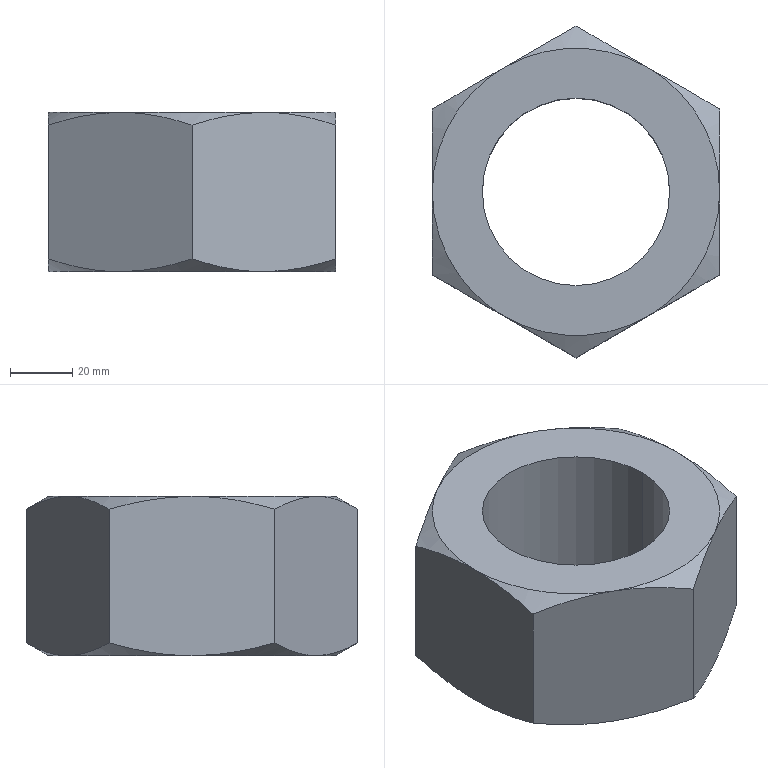Part | SolidWorks | features BaseBody 1 | 1 solid | 22 faces | box 92 x 106.232 x 51 mm | volume 227942 mm3 | cone 12 | plane 8 | cylinder 2 | commonest cylinder face diameters 60 x2
STEP:
#1=CARTESIAN_POINT('',(-30.,0.,51.));
#2=VERTEX_POINT('',#1);
#3=CARTESIAN_POINT('',(30.,0.,51.));
#4=VERTEX_POINT('',#3);
#5=CARTESIAN_POINT('',(0.,0.,51.));
#6=DIRECTION('',(0.,0.,1.));
#7=DIRECTION('',(1.,0.,0.));
#8=AXIS2_PLACEMENT_3D('',#5,#6,#7);
#9=CIRCLE('',#8,30.);
#10=EDGE_CURVE('',#2,#4,#9,.T.);
#11=ORIENTED_EDGE('',*,*,#10,.T.);
#12=CARTESIAN_POINT('',(30.,0.,0.));
#13=VERTEX_POINT('',#12);
#14=CARTESIAN_POINT('',(30.,0.,51.));
#15=DIRECTION('',(0.,0.,-1.));
#16=VECTOR('',#15,1000.);
#17=LINE('',#14,#16);
#18=EDGE_CURVE('',#4,#13,#17,.T.);
#19=ORIENTED_EDGE('',*,*,#18,.T.);
#20=CARTESIAN_POINT('',(-30.,0.,0.));
#21=VERTEX_POINT('',#20);
#22=CARTESIAN_POINT('',(0.,0.,0.));
#23=DIRECTION('',(0.,0.,1.));
#24=DIRECTION('',(1.,0.,0.));
#25=AXIS2_PLACEMENT_3D('',#22,#23,#24);
#26=CIRCLE('',#25,30.);
#27=EDGE_CURVE('',#21,#13,#26,.T.);
#28=ORIENTED_EDGE('',*,*,#27,.F.);
#29=CARTESIAN_POINT('',(-30.,0.,51.));
#30=DIRECTION('',(0.,0.,-1.));
#31=VECTOR('',#30,1000.);
#32=LINE('',#29,#31);
#33=EDGE_CURVE('',#2,#21,#32,.T.);
#34=ORIENTED_EDGE('',*,*,#33,.F.);
#35=EDGE_LOOP('',(#11,#19,#28,#34));
#36=FACE_OUTER_BOUND('',#35,.T.);
#37=CARTESIAN_POINT('',(0.,0.,51.));
#38=DIRECTION('',(0.,0.,-1.));
#39=DIRECTION('',(-1.,0.,0.));
#40=AXIS2_PLACEMENT_3D('',#37,#38,#39);
#41=CYLINDRICAL_SURFACE('',#40,30.);
#42=ADVANCED_FACE('',(#36),#41,.F.);
#43=CARTESIAN_POINT('',(46.,26.558,46.891));
#44=VERTEX_POINT('',#43);
#45=CARTESIAN_POINT('',(23.,39.837,51.));
#46=VERTEX_POINT('',#45);
#47=CARTESIAN_POINT('',(46.,26.558,46.891));
#48=CARTESIAN_POINT('',(42.237,28.73,48.146));
#49=CARTESIAN_POINT('',(38.448,30.919,49.179));
#50=CARTESIAN_POINT('',(32.703,34.235,50.251));
#51=CARTESIAN_POINT('',(30.778,35.346,50.529));
#52=CARTESIAN_POINT('',(26.906,37.582,50.903));
#53=CARTESIAN_POINT('',(24.959,38.706,51.));
#54=CARTESIAN_POINT('',(23.,39.837,51.));
#55=B_SPLINE_CURVE_WITH_KNOTS('',3,(#47,#48,#49,#50,#51,#52,#53,#54),.UNSPECIFIED.,.F.,.F.,(4,2,2,4),(0.000000238,0.01344,0.02015,0.02687),.UNSPECIFIED.);
#56=EDGE_CURVE('',#44,#46,#55,.T.);
#57=ORIENTED_EDGE('',*,*,#56,.F.);
#58=CARTESIAN_POINT('',(46.,26.558,4.109));
#59=VERTEX_POINT('',#58);
#60=CARTESIAN_POINT('',(46.,26.558,51.));
#61=DIRECTION('',(0.,0.,-1.));
#62=VECTOR('',#61,1000.);
#63=LINE('',#60,#62);
#64=EDGE_CURVE('',#44,#59,#63,.T.);
#65=ORIENTED_EDGE('',*,*,#64,.T.);
#66=CARTESIAN_POINT('',(23.,39.837,0.));
#67=VERTEX_POINT('',#66);
#68=CARTESIAN_POINT('',(23.,39.837,0.));
#69=CARTESIAN_POINT('',(23.976,39.274,0.));
#70=CARTESIAN_POINT('',(24.957,38.707,0.0241));
#71=CARTESIAN_POINT('',(26.909,37.58,0.1197));
#72=CARTESIAN_POINT('',(27.882,37.018,0.1911));
#73=CARTESIAN_POINT('',(30.791,35.339,0.4729));
#74=CARTESIAN_POINT('',(32.718,34.227,0.7513));
#75=CARTESIAN_POINT('',(38.462,30.91,1.825));
#76=CARTESIAN_POINT('',(42.247,28.725,2.858));
#77=CARTESIAN_POINT('',(46.,26.558,4.109));
#78=B_SPLINE_CURVE_WITH_KNOTS('',3,(#68,#69,#70,#71,#72,#73,#74,#75,#76,#77),.UNSPECIFIED.,.F.,.F.,(4,2,2,2,4),(0.02687,0.03022,0.03357,0.04026,0.05364),.UNSPECIFIED.);
#79=EDGE_CURVE('',#67,#59,#78,.T.);
#80=ORIENTED_EDGE('',*,*,#79,.F.);
#81=CARTESIAN_POINT('',(0.,53.116,4.109));
#82=VERTEX_POINT('',#81);
#83=CARTESIAN_POINT('',(0.,53.116,4.109));
#84=CARTESIAN_POINT('',(3.763,50.944,2.854));
#85=CARTESIAN_POINT('',(7.552,48.756,1.821));
#86=CARTESIAN_POINT('',(13.297,45.439,0.749));
#87=CARTESIAN_POINT('',(15.222,44.328,0.4714));
#88=CARTESIAN_POINT('',(19.094,42.093,0.09681));
#89=CARTESIAN_POINT('',(21.041,40.968,0.));
#90=CARTESIAN_POINT('',(23.,39.837,0.));
#91=B_SPLINE_CURVE_WITH_KNOTS('',3,(#83,#84,#85,#86,#87,#88,#89,#90),.UNSPECIFIED.,.F.,.F.,(4,2,2,4),(0.000000238,0.01344,0.02015,0.02687),.UNSPECIFIED.);
#92=EDGE_CURVE('',#82,#67,#91,.T.);
#93=ORIENTED_EDGE('',*,*,#92,.F.);
#94=CARTESIAN_POINT('',(0.,53.116,46.891));
#95=VERTEX_POINT('',#94);
#96=CARTESIAN_POINT('',(0.,53.116,51.));
#97=DIRECTION('',(0.,0.,-1.));
#98=VECTOR('',#97,1000.);
#99=LINE('',#96,#98);
#100=EDGE_CURVE('',#95,#82,#99,.T.);
#101=ORIENTED_EDGE('',*,*,#100,.F.);
#102=CARTESIAN_POINT('',(23.,39.837,51.));
#103=CARTESIAN_POINT('',(22.024,40.401,51.));
#104=CARTESIAN_POINT('',(21.043,40.967,50.976));
#105=CARTESIAN_POINT('',(19.091,42.094,50.88));
#106=CARTESIAN_POINT('',(18.118,42.656,50.809));
#107=CARTESIAN_POINT('',(15.209,44.335,50.527));
#108=CARTESIAN_POINT('',(13.282,45.448,50.249));
#109=CARTESIAN_POINT('',(7.538,48.764,49.175));
#110=CARTESIAN_POINT('',(3.753,50.949,48.142));
#111=CARTESIAN_POINT('',(0.,53.116,46.891));
#112=B_SPLINE_CURVE_WITH_KNOTS('',3,(#102,#103,#104,#105,#106,#107,#108,#109,#110,#111),.UNSPECIFIED.,.F.,.F.,(4,2,2,2,4),(0.02687,0.03022,0.03357,0.04026,0.05364),.UNSPECIFIED.);
#113=EDGE_CURVE('',#46,#95,#112,.T.);
#114=ORIENTED_EDGE('',*,*,#113,.F.);
#115=EDGE_LOOP('',(#57,#65,#80,#93,#101,#114));
#116=FACE_OUTER_BOUND('',#115,.T.);
#117=CARTESIAN_POINT('',(46.,26.558,51.));
#118=DIRECTION('',(-0.5,-0.866,0.));
#119=DIRECTION('',(0.866,-0.5,0.));
#120=AXIS2_PLACEMENT_3D('',#117,#118,#119);
#121=PLANE('',#120);
#122=ADVANCED_FACE('',(#116),#121,.F.);
#123=CARTESIAN_POINT('',(-23.,39.837,51.));
#124=VERTEX_POINT('',#123);
#125=CARTESIAN_POINT('',(0.,53.116,46.891));
#126=CARTESIAN_POINT('',(-3.763,50.944,48.146));
#127=CARTESIAN_POINT('',(-7.552,48.756,49.179));
#128=CARTESIAN_POINT('',(-13.297,45.439,50.251));
#129=CARTESIAN_POINT('',(-15.222,44.328,50.529));
#130=CARTESIAN_POINT('',(-19.094,42.093,50.903));
#131=CARTESIAN_POINT('',(-21.041,40.968,51.));
#132=CARTESIAN_POINT('',(-23.,39.837,51.));
#133=B_SPLINE_CURVE_WITH_KNOTS('',3,(#125,#126,#127,#128,#129,#130,#131,#132),.UNSPECIFIED.,.F.,.F.,(4,2,2,4),(0.000000238,0.01344,0.02015,0.02687),.UNSPECIFIED.);
#134=EDGE_CURVE('',#95,#124,#133,.T.);
#135=ORIENTED_EDGE('',*,*,#134,.F.);
#136=ORIENTED_EDGE('',*,*,#100,.T.);
#137=CARTESIAN_POINT('',(-23.,39.837,0.));
#138=VERTEX_POINT('',#137);
#139=CARTESIAN_POINT('',(-23.,39.837,0.));
#140=CARTESIAN_POINT('',(-22.024,40.401,0.));
#141=CARTESIAN_POINT('',(-21.043,40.967,0.0241));
#142=CARTESIAN_POINT('',(-19.091,42.094,0.1197));
#143=CARTESIAN_POINT('',(-18.118,42.656,0.1911));
#144=CARTESIAN_POINT('',(-15.209,44.335,0.4729));
#145=CARTESIAN_POINT('',(-13.282,45.448,0.7513));
#146=CARTESIAN_POINT('',(-7.538,48.764,1.825));
#147=CARTESIAN_POINT('',(-3.753,50.949,2.858));
#148=CARTESIAN_POINT('',(0.,53.116,4.109));
#149=B_SPLINE_CURVE_WITH_KNOTS('',3,(#139,#140,#141,#142,#143,#144,#145,#146,#147,#148),.UNSPECIFIED.,.F.,.F.,(4,2,2,2,4),(0.02687,0.03022,0.03357,0.04026,0.05364),.UNSPECIFIED.);
#150=EDGE_CURVE('',#138,#82,#149,.T.);
#151=ORIENTED_EDGE('',*,*,#150,.F.);
#152=CARTESIAN_POINT('',(-46.,26.558,4.109));
#153=VERTEX_POINT('',#152);
#154=CARTESIAN_POINT('',(-46.,26.558,4.109));
#155=CARTESIAN_POINT('',(-42.237,28.73,2.854));
#156=CARTESIAN_POINT('',(-38.448,30.919,1.821));
#157=CARTESIAN_POINT('',(-32.703,34.235,0.749));
#158=CARTESIAN_POINT('',(-30.778,35.346,0.4714));
#159=CARTESIAN_POINT('',(-26.906,37.582,0.09681));
#160=CARTESIAN_POINT('',(-24.959,38.706,0.));
#161=CARTESIAN_POINT('',(-23.,39.837,0.));
#162=B_SPLINE_CURVE_WITH_KNOTS('',3,(#154,#155,#156,#157,#158,#159,#160,#161),.UNSPECIFIED.,.F.,.F.,(4,2,2,4),(0.000000238,0.01344,0.02015,0.02687),.UNSPECIFIED.);
#163=EDGE_CURVE('',#153,#138,#162,.T.);
#164=ORIENTED_EDGE('',*,*,#163,.F.);
#165=CARTESIAN_POINT('',(-46.,26.558,46.891));
#166=VERTEX_POINT('',#165);
#167=CARTESIAN_POINT('',(-46.,26.558,51.));
#168=DIRECTION('',(0.,0.,-1.));
#169=VECTOR('',#168,1000.);
#170=LINE('',#167,#169);
#171=EDGE_CURVE('',#166,#153,#170,.T.);
#172=ORIENTED_EDGE('',*,*,#171,.F.);
#173=CARTESIAN_POINT('',(-23.,39.837,51.));
#174=CARTESIAN_POINT('',(-23.976,39.274,51.));
#175=CARTESIAN_POINT('',(-24.957,38.707,50.976));
#176=CARTESIAN_POINT('',(-26.909,37.58,50.88));
#177=CARTESIAN_POINT('',(-27.882,37.018,50.809));
#178=CARTESIAN_POINT('',(-30.791,35.339,50.527));
#179=CARTESIAN_POINT('',(-32.718,34.227,50.249));
#180=CARTESIAN_POINT('',(-38.462,30.91,49.175));
#181=CARTESIAN_POINT('',(-42.247,28.725,48.142));
#182=CARTESIAN_POINT('',(-46.,26.558,46.891));
#183=B_SPLINE_CURVE_WITH_KNOTS('',3,(#173,#174,#175,#176,#177,#178,#179,#180,#181,#182),.UNSPECIFIED.,.F.,.F.,(4,2,2,2,4),(0.02687,0.03022,0.03357,0.04026,0.05364),.UNSPECIFIED.);
#184=EDGE_CURVE('',#124,#166,#183,.T.);
#185=ORIENTED_EDGE('',*,*,#184,.F.);
#186=EDGE_LOOP('',(#135,#136,#151,#164,#172,#185));
#187=FACE_OUTER_BOUND('',#186,.T.);
#188=CARTESIAN_POINT('',(0.,53.116,51.));
#189=DIRECTION('',(0.5,-0.866,0.));
#190=DIRECTION('',(0.866,0.5,0.));
#191=AXIS2_PLACEMENT_3D('',#188,#189,#190);
#192=PLANE('',#191);
#193=ADVANCED_FACE('',(#187),#192,.F.);
#194=CARTESIAN_POINT('',(-46.,0.,51.));
#195=VERTEX_POINT('',#194);
#196=CARTESIAN_POINT('',(-46.,26.558,46.891));
#197=CARTESIAN_POINT('',(-46.,22.263,48.131));
#198=CARTESIAN_POINT('',(-46.,17.913,49.163));
#199=CARTESIAN_POINT('',(-46.,11.264,50.243));
#200=CARTESIAN_POINT('',(-46.,9.027,50.524));
#201=CARTESIAN_POINT('',(-46.,4.504,50.904));
#202=CARTESIAN_POINT('',(-46.,2.247,51.));
#203=CARTESIAN_POINT('',(-46.,0.,51.));
#204=B_SPLINE_CURVE_WITH_KNOTS('',3,(#196,#197,#198,#199,#200,#201,#202,#203),.UNSPECIFIED.,.F.,.F.,(4,2,2,4),(0.1492,0.1627,0.1694,0.1761),.UNSPECIFIED.);
#205=EDGE_CURVE('',#166,#195,#204,.T.);
#206=ORIENTED_EDGE('',*,*,#205,.F.);
#207=ORIENTED_EDGE('',*,*,#171,.T.);
#208=CARTESIAN_POINT('',(-46.,0.,0.));
#209=VERTEX_POINT('',#208);
#210=CARTESIAN_POINT('',(-46.,0.,0.));
#211=CARTESIAN_POINT('',(-46.,2.247,0.));
#212=CARTESIAN_POINT('',(-46.,4.504,0.09573));
#213=CARTESIAN_POINT('',(-46.,9.027,0.4757));
#214=CARTESIAN_POINT('',(-46.,11.264,0.757));
#215=CARTESIAN_POINT('',(-46.,17.913,1.837));
#216=CARTESIAN_POINT('',(-46.,22.263,2.869));
#217=CARTESIAN_POINT('',(-46.,26.558,4.109));
#218=B_SPLINE_CURVE_WITH_KNOTS('',3,(#210,#211,#212,#213,#214,#215,#216,#217),.UNSPECIFIED.,.F.,.F.,(4,2,2,4),(0.07541,0.08213,0.08886,0.1023),.UNSPECIFIED.);
#219=EDGE_CURVE('',#209,#153,#218,.T.);
#220=ORIENTED_EDGE('',*,*,#219,.F.);
#221=CARTESIAN_POINT('',(-46.,-26.558,4.109));
#222=VERTEX_POINT('',#221);
#223=CARTESIAN_POINT('',(-46.,-26.558,4.109));
#224=CARTESIAN_POINT('',(-46.,-25.477,3.797));
#225=CARTESIAN_POINT('',(-46.,-24.392,3.497));
#226=CARTESIAN_POINT('',(-46.,-22.209,2.928));
#227=CARTESIAN_POINT('',(-46.,-21.11,2.657));
#228=CARTESIAN_POINT('',(-46.,-17.806,1.896));
#229=CARTESIAN_POINT('',(-46.,-15.597,1.458));
#230=CARTESIAN_POINT('',(-46.,-11.166,0.7436));
#231=CARTESIAN_POINT('',(-46.,-8.943,0.4673));
#232=CARTESIAN_POINT('',(-46.,-4.483,0.09541));
#233=CARTESIAN_POINT('',(-46.,-2.246,0.));
#234=CARTESIAN_POINT('',(-46.,0.,0.));
#235=B_SPLINE_CURVE_WITH_KNOTS('',3,(#223,#224,#225,#226,#227,#228,#229,#230,#231,#232,#233,#234),.UNSPECIFIED.,.F.,.F.,(4,2,2,2,2,4),(0.04853,0.05189,0.05525,0.06197,0.06869,0.07541),.UNSPECIFIED.);
#236=EDGE_CURVE('',#222,#209,#235,.T.);
#237=ORIENTED_EDGE('',*,*,#236,.F.);
#238=CARTESIAN_POINT('',(-46.,-26.558,46.891));
#239=VERTEX_POINT('',#238);
#240=CARTESIAN_POINT('',(-46.,-26.558,51.));
#241=DIRECTION('',(0.,0.,-1.));
#242=VECTOR('',#241,1000.);
#243=LINE('',#240,#242);
#244=EDGE_CURVE('',#239,#222,#243,.T.);
#245=ORIENTED_EDGE('',*,*,#244,.F.);
#246=CARTESIAN_POINT('',(-46.,0.,51.));
#247=CARTESIAN_POINT('',(-46.,-2.246,51.));
#248=CARTESIAN_POINT('',(-46.,-4.483,50.905));
#249=CARTESIAN_POINT('',(-46.,-8.943,50.533));
#250=CARTESIAN_POINT('',(-46.,-11.166,50.256));
#251=CARTESIAN_POINT('',(-46.,-15.597,49.542));
#252=CARTESIAN_POINT('',(-46.,-17.806,49.104));
#253=CARTESIAN_POINT('',(-46.,-21.11,48.343));
#254=CARTESIAN_POINT('',(-46.,-22.209,48.072));
#255=CARTESIAN_POINT('',(-46.,-24.392,47.503));
#256=CARTESIAN_POINT('',(-46.,-25.477,47.203));
#257=CARTESIAN_POINT('',(-46.,-26.558,46.891));
#258=B_SPLINE_CURVE_WITH_KNOTS('',3,(#246,#247,#248,#249,#250,#251,#252,#253,#254,#255,#256,#257),.UNSPECIFIED.,.F.,.F.,(4,2,2,2,2,4),(0.1761,0.1828,0.1895,0.1963,0.1996,0.203),.UNSPECIFIED.);
#259=EDGE_CURVE('',#195,#239,#258,.T.);
#260=ORIENTED_EDGE('',*,*,#259,.F.);
#261=EDGE_LOOP('',(#206,#207,#220,#237,#245,#260));
#262=FACE_OUTER_BOUND('',#261,.T.);
#263=CARTESIAN_POINT('',(-46.,26.558,51.));
#264=DIRECTION('',(1.,0.,0.));
#265=DIRECTION('',(0.,1.,0.));
#266=AXIS2_PLACEMENT_3D('',#263,#264,#265);
#267=PLANE('',#266);
#268=ADVANCED_FACE('',(#262),#267,.F.);
#269=CARTESIAN_POINT('',(-23.,-39.837,51.));
#270=VERTEX_POINT('',#269);
#271=CARTESIAN_POINT('',(-46.,-26.558,46.891));
#272=CARTESIAN_POINT('',(-42.237,-28.73,48.146));
#273=CARTESIAN_POINT('',(-38.448,-30.919,49.179));
#274=CARTESIAN_POINT('',(-32.703,-34.235,50.251));
#275=CARTESIAN_POINT('',(-30.778,-35.346,50.529));
#276=CARTESIAN_POINT('',(-26.906,-37.582,50.903));
#277=CARTESIAN_POINT('',(-24.959,-38.706,51.));
#278=CARTESIAN_POINT('',(-23.,-39.837,51.));
#279=B_SPLINE_CURVE_WITH_KNOTS('',3,(#271,#272,#273,#274,#275,#276,#277,#278),.UNSPECIFIED.,.F.,.F.,(4,2,2,4),(0.000000238,0.01344,0.02015,0.02687),.UNSPECIFIED.);
#280=EDGE_CURVE('',#239,#270,#279,.T.);
#281=ORIENTED_EDGE('',*,*,#280,.F.);
#282=ORIENTED_EDGE('',*,*,#244,.T.);
#283=CARTESIAN_POINT('',(-23.,-39.837,0.));
#284=VERTEX_POINT('',#283);
#285=CARTESIAN_POINT('',(-23.,-39.837,0.));
#286=CARTESIAN_POINT('',(-23.976,-39.274,0.));
#287=CARTESIAN_POINT('',(-24.957,-38.707,0.0241));
#288=CARTESIAN_POINT('',(-26.909,-37.58,0.1197));
#289=CARTESIAN_POINT('',(-27.882,-37.018,0.1911));
#290=CARTESIAN_POINT('',(-30.791,-35.339,0.4729));
#291=CARTESIAN_POINT('',(-32.718,-34.227,0.7513));
#292=CARTESIAN_POINT('',(-38.462,-30.91,1.825));
#293=CARTESIAN_POINT('',(-42.247,-28.725,2.858));
#294=CARTESIAN_POINT('',(-46.,-26.558,4.109));
#295=B_SPLINE_CURVE_WITH_KNOTS('',3,(#285,#286,#287,#288,#289,#290,#291,#292,#293,#294),.UNSPECIFIED.,.F.,.F.,(4,2,2,2,4),(0.02687,0.03022,0.03357,0.04026,0.05364),.UNSPECIFIED.);
#296=EDGE_CURVE('',#284,#222,#295,.T.);
#297=ORIENTED_EDGE('',*,*,#296,.F.);
#298=CARTESIAN_POINT('',(0.,-53.116,4.109));
#299=VERTEX_POINT('',#298);
#300=CARTESIAN_POINT('',(0.,-53.116,4.109));
#301=CARTESIAN_POINT('',(-3.763,-50.944,2.854));
#302=CARTESIAN_POINT('',(-7.552,-48.756,1.821));
#303=CARTESIAN_POINT('',(-13.297,-45.439,0.749));
#304=CARTESIAN_POINT('',(-15.222,-44.328,0.4714));
#305=CARTESIAN_POINT('',(-19.094,-42.093,0.09681));
#306=CARTESIAN_POINT('',(-21.041,-40.968,0.));
#307=CARTESIAN_POINT('',(-23.,-39.837,0.));
#308=B_SPLINE_CURVE_WITH_KNOTS('',3,(#300,#301,#302,#303,#304,#305,#306,#307),.UNSPECIFIED.,.F.,.F.,(4,2,2,4),(0.000000238,0.01344,0.02015,0.02687),.UNSPECIFIED.);
#309=EDGE_CURVE('',#299,#284,#308,.T.);
#310=ORIENTED_EDGE('',*,*,#309,.F.);
#311=CARTESIAN_POINT('',(0.,-53.116,46.891));
#312=VERTEX_POINT('',#311);
#313=CARTESIAN_POINT('',(0.,-53.116,51.));
#314=DIRECTION('',(0.,0.,-1.));
#315=VECTOR('',#314,1000.);
#316=LINE('',#313,#315);
#317=EDGE_CURVE('',#312,#299,#316,.T.);
#318=ORIENTED_EDGE('',*,*,#317,.F.);
#319=CARTESIAN_POINT('',(-23.,-39.837,51.));
#320=CARTESIAN_POINT('',(-22.024,-40.401,51.));
#321=CARTESIAN_POINT('',(-21.043,-40.967,50.976));
#322=CARTESIAN_POINT('',(-19.091,-42.094,50.88));
#323=CARTESIAN_POINT('',(-18.118,-42.656,50.809));
#324=CARTESIAN_POINT('',(-15.209,-44.335,50.527));
#325=CARTESIAN_POINT('',(-13.282,-45.448,50.249));
#326=CARTESIAN_POINT('',(-7.538,-48.764,49.175));
#327=CARTESIAN_POINT('',(-3.753,-50.949,48.142));
#328=CARTESIAN_POINT('',(0.,-53.116,46.891));
#329=B_SPLINE_CURVE_WITH_KNOTS('',3,(#319,#320,#321,#322,#323,#324,#325,#326,#327,#328),.UNSPECIFIED.,.F.,.F.,(4,2,2,2,4),(0.02687,0.03022,0.03357,0.04026,0.05364),.UNSPECIFIED.);
#330=EDGE_CURVE('',#270,#312,#329,.T.);
#331=ORIENTED_EDGE('',*,*,#330,.F.);
#332=EDGE_LOOP('',(#281,#282,#297,#310,#318,#331));
#333=FACE_OUTER_BOUND('',#332,.T.);
#334=CARTESIAN_POINT('',(-46.,-26.558,51.));
#335=DIRECTION('',(0.5,0.866,0.));
#336=DIRECTION('',(-0.866,0.5,0.));
#337=AXIS2_PLACEMENT_3D('',#334,#335,#336);
#338=PLANE('',#337);
#339=ADVANCED_FACE('',(#333),#338,.F.);
#340=CARTESIAN_POINT('',(23.,-39.837,51.));
#341=VERTEX_POINT('',#340);
#342=CARTESIAN_POINT('',(0.,-53.116,46.891));
#343=CARTESIAN_POINT('',(3.763,-50.944,48.146));
#344=CARTESIAN_POINT('',(7.552,-48.756,49.179));
#345=CARTESIAN_POINT('',(13.297,-45.439,50.251));
#346=CARTESIAN_POINT('',(15.222,-44.328,50.529));
#347=CARTESIAN_POINT('',(19.094,-42.093,50.903));
#348=CARTESIAN_POINT('',(21.041,-40.968,51.));
#349=CARTESIAN_POINT('',(23.,-39.837,51.));
#350=B_SPLINE_CURVE_WITH_KNOTS('',3,(#342,#343,#344,#345,#346,#347,#348,#349),.UNSPECIFIED.,.F.,.F.,(4,2,2,4),(0.000000238,0.01344,0.02015,0.02687),.UNSPECIFIED.);
#351=EDGE_CURVE('',#312,#341,#350,.T.);
#352=ORIENTED_EDGE('',*,*,#351,.F.);
#353=ORIENTED_EDGE('',*,*,#317,.T.);
#354=CARTESIAN_POINT('',(23.,-39.837,0.));
#355=VERTEX_POINT('',#354);
#356=CARTESIAN_POINT('',(23.,-39.837,0.));
#357=CARTESIAN_POINT('',(22.024,-40.401,0.));
#358=CARTESIAN_POINT('',(21.043,-40.967,0.0241));
#359=CARTESIAN_POINT('',(19.091,-42.094,0.1197));
#360=CARTESIAN_POINT('',(18.118,-42.656,0.1911));
#361=CARTESIAN_POINT('',(15.209,-44.335,0.4729));
#362=CARTESIAN_POINT('',(13.282,-45.448,0.7513));
#363=CARTESIAN_POINT('',(7.538,-48.764,1.825));
#364=CARTESIAN_POINT('',(3.753,-50.949,2.858));
#365=CARTESIAN_POINT('',(0.,-53.116,4.109));
#366=B_SPLINE_CURVE_WITH_KNOTS('',3,(#356,#357,#358,#359,#360,#361,#362,#363,#364,#365),.UNSPECIFIED.,.F.,.F.,(4,2,2,2,4),(0.02687,0.03022,0.03357,0.04026,0.05364),.UNSPECIFIED.);
#367=EDGE_CURVE('',#355,#299,#366,.T.);
#368=ORIENTED_EDGE('',*,*,#367,.F.);
#369=CARTESIAN_POINT('',(46.,-26.558,4.109));
#370=VERTEX_POINT('',#369);
#371=CARTESIAN_POINT('',(46.,-26.558,4.109));
#372=CARTESIAN_POINT('',(42.237,-28.73,2.854));
#373=CARTESIAN_POINT('',(38.448,-30.919,1.821));
#374=CARTESIAN_POINT('',(32.703,-34.235,0.749));
#375=CARTESIAN_POINT('',(30.778,-35.346,0.4714));
#376=CARTESIAN_POINT('',(26.906,-37.582,0.09681));
#377=CARTESIAN_POINT('',(24.959,-38.706,0.));
#378=CARTESIAN_POINT('',(23.,-39.837,0.));
#379=B_SPLINE_CURVE_WITH_KNOTS('',3,(#371,#372,#373,#374,#375,#376,#377,#378),.UNSPECIFIED.,.F.,.F.,(4,2,2,4),(0.000000238,0.01344,0.02015,0.02687),.UNSPECIFIED.);
#380=EDGE_CURVE('',#370,#355,#379,.T.);
#381=ORIENTED_EDGE('',*,*,#380,.F.);
#382=CARTESIAN_POINT('',(46.,-26.558,46.891));
#383=VERTEX_POINT('',#382);
#384=CARTESIAN_POINT('',(46.,-26.558,51.));
#385=DIRECTION('',(0.,0.,-1.));
#386=VECTOR('',#385,1000.);
#387=LINE('',#384,#386);
#388=EDGE_CURVE('',#383,#370,#387,.T.);
#389=ORIENTED_EDGE('',*,*,#388,.F.);
#390=CARTESIAN_POINT('',(23.,-39.837,51.));
#391=CARTESIAN_POINT('',(23.976,-39.274,51.));
#392=CARTESIAN_POINT('',(24.957,-38.707,50.976));
#393=CARTESIAN_POINT('',(26.909,-37.58,50.88));
#394=CARTESIAN_POINT('',(27.882,-37.018,50.809));
#395=CARTESIAN_POINT('',(30.791,-35.339,50.527));
#396=CARTESIAN_POINT('',(32.718,-34.227,50.249));
#397=CARTESIAN_POINT('',(38.462,-30.91,49.175));
#398=CARTESIAN_POINT('',(42.247,-28.725,48.142));
#399=CARTESIAN_POINT('',(46.,-26.558,46.891));
#400=B_SPLINE_CURVE_WITH_KNOTS('',3,(#390,#391,#392,#393,#394,#395,#396,#397,#398,#399),.UNSPECIFIED.,.F.,.F.,(4,2,2,2,4),(0.02687,0.03022,0.03357,0.04026,0.05364),.UNSPECIFIED.);
#401=EDGE_CURVE('',#341,#383,#400,.T.);
#402=ORIENTED_EDGE('',*,*,#401,.F.);
#403=EDGE_LOOP('',(#352,#353,#368,#381,#389,#402));
#404=FACE_OUTER_BOUND('',#403,.T.);
#405=CARTESIAN_POINT('',(0.,-53.116,51.));
#406=DIRECTION('',(-0.5,0.866,0.));
#407=DIRECTION('',(-0.866,-0.5,0.));
#408=AXIS2_PLACEMENT_3D('',#405,#406,#407);
#409=PLANE('',#408);
#410=ADVANCED_FACE('',(#404),#409,.F.);
#411=CARTESIAN_POINT('',(46.,0.,51.));
#412=VERTEX_POINT('',#411);
#413=CARTESIAN_POINT('',(46.,-26.558,46.891));
#414=CARTESIAN_POINT('',(46.,-25.477,47.203));
#415=CARTESIAN_POINT('',(46.,-24.392,47.503));
#416=CARTESIAN_POINT('',(46.,-22.209,48.072));
#417=CARTESIAN_POINT('',(46.,-21.11,48.343));
#418=CARTESIAN_POINT('',(46.,-17.806,49.104));
#419=CARTESIAN_POINT('',(46.,-15.597,49.542));
#420=CARTESIAN_POINT('',(46.,-11.166,50.256));
#421=CARTESIAN_POINT('',(46.,-8.943,50.533));
#422=CARTESIAN_POINT('',(46.,-4.483,50.905));
#423=CARTESIAN_POINT('',(46.,-2.246,51.));
#424=CARTESIAN_POINT('',(46.,0.,51.));
#425=B_SPLINE_CURVE_WITH_KNOTS('',3,(#413,#414,#415,#416,#417,#418,#419,#420,#421,#422,#423,#424),.UNSPECIFIED.,.F.,.F.,(4,2,2,2,2,4),(0.04853,0.05189,0.05525,0.06197,0.06869,0.07541),.UNSPECIFIED.);
#426=EDGE_CURVE('',#383,#412,#425,.T.);
#427=ORIENTED_EDGE('',*,*,#426,.F.);
#428=ORIENTED_EDGE('',*,*,#388,.T.);
#429=CARTESIAN_POINT('',(46.,0.,0.));
#430=VERTEX_POINT('',#429);
#431=CARTESIAN_POINT('',(46.,0.,0.));
#432=CARTESIAN_POINT('',(46.,-2.246,0.));
#433=CARTESIAN_POINT('',(46.,-4.483,0.09541));
#434=CARTESIAN_POINT('',(46.,-8.943,0.4673));
#435=CARTESIAN_POINT('',(46.,-11.166,0.7436));
#436=CARTESIAN_POINT('',(46.,-15.597,1.458));
#437=CARTESIAN_POINT('',(46.,-17.806,1.896));
#438=CARTESIAN_POINT('',(46.,-21.11,2.657));
#439=CARTESIAN_POINT('',(46.,-22.209,2.928));
#440=CARTESIAN_POINT('',(46.,-24.392,3.497));
#441=CARTESIAN_POINT('',(46.,-25.477,3.797));
#442=CARTESIAN_POINT('',(46.,-26.558,4.109));
#443=B_SPLINE_CURVE_WITH_KNOTS('',3,(#431,#432,#433,#434,#435,#436,#437,#438,#439,#440,#441,#442),.UNSPECIFIED.,.F.,.F.,(4,2,2,2,2,4),(0.1761,0.1828,0.1895,0.1963,0.1996,0.203),.UNSPECIFIED.);
#444=EDGE_CURVE('',#430,#370,#443,.T.);
#445=ORIENTED_EDGE('',*,*,#444,.F.);
#446=CARTESIAN_POINT('',(46.,26.558,4.109));
#447=CARTESIAN_POINT('',(46.,22.263,2.869));
#448=CARTESIAN_POINT('',(46.,17.913,1.837));
#449=CARTESIAN_POINT('',(46.,11.264,0.757));
#450=CARTESIAN_POINT('',(46.,9.027,0.4757));
#451=CARTESIAN_POINT('',(46.,4.504,0.09573));
#452=CARTESIAN_POINT('',(46.,2.247,0.));
#453=CARTESIAN_POINT('',(46.,0.,0.));
#454=B_SPLINE_CURVE_WITH_KNOTS('',3,(#446,#447,#448,#449,#450,#451,#452,#453),.UNSPECIFIED.,.F.,.F.,(4,2,2,4),(0.1492,0.1627,0.1694,0.1761),.UNSPECIFIED.);
#455=EDGE_CURVE('',#59,#430,#454,.T.);
#456=ORIENTED_EDGE('',*,*,#455,.F.);
#457=ORIENTED_EDGE('',*,*,#64,.F.);
#458=CARTESIAN_POINT('',(46.,0.,51.));
#459=CARTESIAN_POINT('',(46.,2.247,51.));
#460=CARTESIAN_POINT('',(46.,4.504,50.904));
#461=CARTESIAN_POINT('',(46.,9.027,50.524));
#462=CARTESIAN_POINT('',(46.,11.264,50.243));
#463=CARTESIAN_POINT('',(46.,17.913,49.163));
#464=CARTESIAN_POINT('',(46.,22.263,48.131));
#465=CARTESIAN_POINT('',(46.,26.558,46.891));
#466=B_SPLINE_CURVE_WITH_KNOTS('',3,(#458,#459,#460,#461,#462,#463,#464,#465),.UNSPECIFIED.,.F.,.F.,(4,2,2,4),(0.07541,0.08213,0.08886,0.1023),.UNSPECIFIED.);
#467=EDGE_CURVE('',#412,#44,#466,.T.);
#468=ORIENTED_EDGE('',*,*,#467,.F.);
#469=EDGE_LOOP('',(#427,#428,#445,#456,#457,#468));
#470=FACE_OUTER_BOUND('',#469,.T.);
#471=CARTESIAN_POINT('',(46.,-26.558,51.));
#472=DIRECTION('',(-1.,0.,0.));
#473=DIRECTION('',(0.,-1.,0.));
#474=AXIS2_PLACEMENT_3D('',#471,#472,#473);
#475=PLANE('',#474);
#476=ADVANCED_FACE('',(#470),#475,.F.);
#477=ORIENTED_EDGE('',*,*,#10,.F.);
#478=CARTESIAN_POINT('',(0.,0.,51.));
#479=DIRECTION('',(0.,0.,1.));
#480=DIRECTION('',(1.,0.,0.));
#481=AXIS2_PLACEMENT_3D('',#478,#479,#480);
#482=CIRCLE('',#481,30.);
#483=EDGE_CURVE('',#4,#2,#482,.T.);
#484=ORIENTED_EDGE('',*,*,#483,.F.);
#485=EDGE_LOOP('',(#477,#484));
#486=FACE_BOUND('',#485,.T.);
#487=CARTESIAN_POINT('',(0.,0.,51.));
#488=DIRECTION('',(0.,0.,1.));
#489=DIRECTION('',(1.,0.,0.));
#490=AXIS2_PLACEMENT_3D('',#487,#488,#489);
#491=CIRCLE('',#490,46.);
#492=EDGE_CURVE('',#341,#412,#491,.T.);
#493=ORIENTED_EDGE('',*,*,#492,.T.);
#494=CARTESIAN_POINT('',(0.,0.,51.));
#495=DIRECTION('',(0.,0.,1.));
#496=DIRECTION('',(1.,0.,0.));
#497=AXIS2_PLACEMENT_3D('',#494,#495,#496);
#498=CIRCLE('',#497,46.);
#499=EDGE_CURVE('',#412,#46,#498,.T.);
#500=ORIENTED_EDGE('',*,*,#499,.T.);
#501=CARTESIAN_POINT('',(0.,0.,51.));
#502=DIRECTION('',(0.,0.,1.));
#503=DIRECTION('',(1.,0.,0.));
#504=AXIS2_PLACEMENT_3D('',#501,#502,#503);
#505=CIRCLE('',#504,46.);
#506=EDGE_CURVE('',#46,#124,#505,.T.);
#507=ORIENTED_EDGE('',*,*,#506,.T.);
#508=CARTESIAN_POINT('',(0.,0.,51.));
#509=DIRECTION('',(0.,0.,1.));
#510=DIRECTION('',(1.,0.,0.));
#511=AXIS2_PLACEMENT_3D('',#508,#509,#510);
#512=CIRCLE('',#511,46.);
#513=EDGE_CURVE('',#124,#195,#512,.T.);
#514=ORIENTED_EDGE('',*,*,#513,.T.);
#515=CARTESIAN_POINT('',(0.,0.,51.));
#516=DIRECTION('',(0.,0.,1.));
#517=DIRECTION('',(1.,0.,0.));
#518=AXIS2_PLACEMENT_3D('',#515,#516,#517);
#519=CIRCLE('',#518,46.);
#520=EDGE_CURVE('',#195,#270,#519,.T.);
#521=ORIENTED_EDGE('',*,*,#520,.T.);
#522=CARTESIAN_POINT('',(0.,0.,51.));
#523=DIRECTION('',(0.,0.,1.));
#524=DIRECTION('',(1.,0.,0.));
#525=AXIS2_PLACEMENT_3D('',#522,#523,#524);
#526=CIRCLE('',#525,46.);
#527=EDGE_CURVE('',#270,#341,#526,.T.);
#528=ORIENTED_EDGE('',*,*,#527,.T.);
#529=EDGE_LOOP('',(#493,#500,#507,#514,#521,#528));
#530=FACE_OUTER_BOUND('',#529,.T.);
#531=CARTESIAN_POINT('',(-46.,79.674,51.));
#532=DIRECTION('',(0.,0.,1.));
#533=DIRECTION('',(1.,0.,0.));
#534=AXIS2_PLACEMENT_3D('',#531,#532,#533);
#535=PLANE('',#534);
#536=ADVANCED_FACE('',(#486,#530),#535,.T.);
#537=ORIENTED_EDGE('',*,*,#27,.T.);
#538=CARTESIAN_POINT('',(0.,0.,0.));
#539=DIRECTION('',(0.,0.,1.));
#540=DIRECTION('',(1.,0.,0.));
#541=AXIS2_PLACEMENT_3D('',#538,#539,#540);
#542=CIRCLE('',#541,30.);
#543=EDGE_CURVE('',#13,#21,#542,.T.);
#544=ORIENTED_EDGE('',*,*,#543,.T.);
#545=EDGE_LOOP('',(#537,#544));
#546=FACE_BOUND('',#545,.T.);
#547=CARTESIAN_POINT('',(0.,0.,0.));
#548=DIRECTION('',(0.,0.,-1.));
#549=DIRECTION('',(-1.,0.,0.));
#550=AXIS2_PLACEMENT_3D('',#547,#548,#549);
#551=CIRCLE('',#550,46.);
#552=EDGE_CURVE('',#67,#430,#551,.T.);
#553=ORIENTED_EDGE('',*,*,#552,.T.);
#554=CARTESIAN_POINT('',(0.,0.,0.));
#555=DIRECTION('',(0.,0.,-1.));
#556=DIRECTION('',(-1.,0.,0.));
#557=AXIS2_PLACEMENT_3D('',#554,#555,#556);
#558=CIRCLE('',#557,46.);
#559=EDGE_CURVE('',#430,#355,#558,.T.);
#560=ORIENTED_EDGE('',*,*,#559,.T.);
#561=CARTESIAN_POINT('',(0.,0.,0.));
#562=DIRECTION('',(0.,0.,-1.));
#563=DIRECTION('',(-1.,0.,0.));
#564=AXIS2_PLACEMENT_3D('',#561,#562,#563);
#565=CIRCLE('',#564,46.);
#566=EDGE_CURVE('',#355,#284,#565,.T.);
#567=ORIENTED_EDGE('',*,*,#566,.T.);
#568=CARTESIAN_POINT('',(0.,0.,0.));
#569=DIRECTION('',(0.,0.,-1.));
#570=DIRECTION('',(-1.,0.,0.));
#571=AXIS2_PLACEMENT_3D('',#568,#569,#570);
#572=CIRCLE('',#571,46.);
#573=EDGE_CURVE('',#284,#209,#572,.T.);
#574=ORIENTED_EDGE('',*,*,#573,.T.);
#575=CARTESIAN_POINT('',(0.,0.,0.));
#576=DIRECTION('',(0.,0.,-1.));
#577=DIRECTION('',(-1.,0.,0.));
#578=AXIS2_PLACEMENT_3D('',#575,#576,#577);
#579=CIRCLE('',#578,46.);
#580=EDGE_CURVE('',#209,#138,#579,.T.);
#581=ORIENTED_EDGE('',*,*,#580,.T.);
#582=CARTESIAN_POINT('',(0.,0.,0.));
#583=DIRECTION('',(0.,0.,-1.));
#584=DIRECTION('',(-1.,0.,0.));
#585=AXIS2_PLACEMENT_3D('',#582,#583,#584);
#586=CIRCLE('',#585,46.);
#587=EDGE_CURVE('',#138,#67,#586,.T.);
#588=ORIENTED_EDGE('',*,*,#587,.T.);
#589=EDGE_LOOP('',(#553,#560,#567,#574,#581,#588));
#590=FACE_OUTER_BOUND('',#589,.T.);
#591=CARTESIAN_POINT('',(-46.,79.674,0.));
#592=DIRECTION('',(0.,0.,1.));
#593=DIRECTION('',(1.,0.,0.));
#594=AXIS2_PLACEMENT_3D('',#591,#592,#593);
#595=PLANE('',#594);
#596=ADVANCED_FACE('',(#546,#590),#595,.F.);
#597=ORIENTED_EDGE('',*,*,#18,.F.);
#598=ORIENTED_EDGE('',*,*,#483,.T.);
#599=ORIENTED_EDGE('',*,*,#33,.T.);
#600=ORIENTED_EDGE('',*,*,#543,.F.);
#601=EDGE_LOOP('',(#597,#598,#599,#600));
#602=FACE_OUTER_BOUND('',#601,.T.);
#603=CARTESIAN_POINT('',(0.,0.,51.));
#604=DIRECTION('',(0.,0.,-1.));
#605=DIRECTION('',(-1.,0.,0.));
#606=AXIS2_PLACEMENT_3D('',#603,#604,#605);
#607=CYLINDRICAL_SURFACE('',#606,30.);
#608=ADVANCED_FACE('',(#602),#607,.F.);
#609=ORIENTED_EDGE('',*,*,#380,.T.);
#610=ORIENTED_EDGE('',*,*,#559,.F.);
#611=ORIENTED_EDGE('',*,*,#444,.T.);
#612=EDGE_LOOP('',(#609,#610,#611));
#613=FACE_OUTER_BOUND('',#612,.T.);
#614=CARTESIAN_POINT('',(0.,0.,0.));
#615=DIRECTION('',(0.,0.,1.));
#616=DIRECTION('',(-1.,0.,0.));
#617=AXIS2_PLACEMENT_3D('',#614,#615,#616);
#618=CONICAL_SURFACE('',#617,46.,1.047);
#619=ADVANCED_FACE('',(#613),#618,.T.);
#620=ORIENTED_EDGE('',*,*,#79,.T.);
#621=ORIENTED_EDGE('',*,*,#455,.T.);
#622=ORIENTED_EDGE('',*,*,#552,.F.);
#623=EDGE_LOOP('',(#620,#621,#622));
#624=FACE_OUTER_BOUND('',#623,.T.);
#625=CARTESIAN_POINT('',(0.,0.,0.));
#626=DIRECTION('',(0.,0.,1.));
#627=DIRECTION('',(-1.,0.,0.));
#628=AXIS2_PLACEMENT_3D('',#625,#626,#627);
#629=CONICAL_SURFACE('',#628,46.,1.047);
#630=ADVANCED_FACE('',(#624),#629,.T.);
#631=ORIENTED_EDGE('',*,*,#309,.T.);
#632=ORIENTED_EDGE('',*,*,#566,.F.);
#633=ORIENTED_EDGE('',*,*,#367,.T.);
#634=EDGE_LOOP('',(#631,#632,#633));
#635=FACE_OUTER_BOUND('',#634,.T.);
#636=CARTESIAN_POINT('',(0.,0.,0.));
#637=DIRECTION('',(0.,0.,1.));
#638=DIRECTION('',(-1.,0.,0.));
#639=AXIS2_PLACEMENT_3D('',#636,#637,#638);
#640=CONICAL_SURFACE('',#639,46.,1.047);
#641=ADVANCED_FACE('',(#635),#640,.T.);
#642=ORIENTED_EDGE('',*,*,#236,.T.);
#643=ORIENTED_EDGE('',*,*,#573,.F.);
#644=ORIENTED_EDGE('',*,*,#296,.T.);
#645=EDGE_LOOP('',(#642,#643,#644));
#646=FACE_OUTER_BOUND('',#645,.T.);
#647=CARTESIAN_POINT('',(0.,0.,0.));
#648=DIRECTION('',(0.,0.,1.));
#649=DIRECTION('',(-1.,0.,0.));
#650=AXIS2_PLACEMENT_3D('',#647,#648,#649);
#651=CONICAL_SURFACE('',#650,46.,1.047);
#652=ADVANCED_FACE('',(#646),#651,.T.);
#653=ORIENTED_EDGE('',*,*,#219,.T.);
#654=ORIENTED_EDGE('',*,*,#163,.T.);
#655=ORIENTED_EDGE('',*,*,#580,.F.);
#656=EDGE_LOOP('',(#653,#654,#655));
#657=FACE_OUTER_BOUND('',#656,.T.);
#658=CARTESIAN_POINT('',(0.,0.,0.));
#659=DIRECTION('',(0.,0.,1.));
#660=DIRECTION('',(-1.,0.,0.));
#661=AXIS2_PLACEMENT_3D('',#658,#659,#660);
#662=CONICAL_SURFACE('',#661,46.,1.047);
#663=ADVANCED_FACE('',(#657),#662,.T.);
#664=ORIENTED_EDGE('',*,*,#150,.T.);
#665=ORIENTED_EDGE('',*,*,#92,.T.);
#666=ORIENTED_EDGE('',*,*,#587,.F.);
#667=EDGE_LOOP('',(#664,#665,#666));
#668=FACE_OUTER_BOUND('',#667,.T.);
#669=CARTESIAN_POINT('',(0.,0.,0.));
#670=DIRECTION('',(0.,0.,1.));
#671=DIRECTION('',(-1.,0.,0.));
#672=AXIS2_PLACEMENT_3D('',#669,#670,#671);
#673=CONICAL_SURFACE('',#672,46.,1.047);
#674=ADVANCED_FACE('',(#668),#673,.T.);
#675=ORIENTED_EDGE('',*,*,#401,.T.);
#676=ORIENTED_EDGE('',*,*,#426,.T.);
#677=ORIENTED_EDGE('',*,*,#492,.F.);
#678=EDGE_LOOP('',(#675,#676,#677));
#679=FACE_OUTER_BOUND('',#678,.T.);
#680=CARTESIAN_POINT('',(0.,0.,51.));
#681=DIRECTION('',(0.,0.,-1.));
#682=DIRECTION('',(1.,0.,0.));
#683=AXIS2_PLACEMENT_3D('',#680,#681,#682);
#684=CONICAL_SURFACE('',#683,46.,1.047);
#685=ADVANCED_FACE('',(#679),#684,.T.);
#686=ORIENTED_EDGE('',*,*,#330,.T.);
#687=ORIENTED_EDGE('',*,*,#351,.T.);
#688=ORIENTED_EDGE('',*,*,#527,.F.);
#689=EDGE_LOOP('',(#686,#687,#688));
#690=FACE_OUTER_BOUND('',#689,.T.);
#691=CARTESIAN_POINT('',(0.,0.,51.));
#692=DIRECTION('',(0.,0.,-1.));
#693=DIRECTION('',(1.,0.,0.));
#694=AXIS2_PLACEMENT_3D('',#691,#692,#693);
#695=CONICAL_SURFACE('',#694,46.,1.047);
#696=ADVANCED_FACE('',(#690),#695,.T.);
#697=ORIENTED_EDGE('',*,*,#259,.T.);
#698=ORIENTED_EDGE('',*,*,#280,.T.);
#699=ORIENTED_EDGE('',*,*,#520,.F.);
#700=EDGE_LOOP('',(#697,#698,#699));
#701=FACE_OUTER_BOUND('',#700,.T.);
#702=CARTESIAN_POINT('',(0.,0.,51.));
#703=DIRECTION('',(0.,0.,-1.));
#704=DIRECTION('',(1.,0.,0.));
#705=AXIS2_PLACEMENT_3D('',#702,#703,#704);
#706=CONICAL_SURFACE('',#705,46.,1.047);
#707=ADVANCED_FACE('',(#701),#706,.T.);
#708=ORIENTED_EDGE('',*,*,#184,.T.);
#709=ORIENTED_EDGE('',*,*,#205,.T.);
#710=ORIENTED_EDGE('',*,*,#513,.F.);
#711=EDGE_LOOP('',(#708,#709,#710));
#712=FACE_OUTER_BOUND('',#711,.T.);
#713=CARTESIAN_POINT('',(0.,0.,51.));
#714=DIRECTION('',(0.,0.,-1.));
#715=DIRECTION('',(1.,0.,0.));
#716=AXIS2_PLACEMENT_3D('',#713,#714,#715);
#717=CONICAL_SURFACE('',#716,46.,1.047);
#718=ADVANCED_FACE('',(#712),#717,.T.);
#719=ORIENTED_EDGE('',*,*,#113,.T.);
#720=ORIENTED_EDGE('',*,*,#134,.T.);
#721=ORIENTED_EDGE('',*,*,#506,.F.);
#722=EDGE_LOOP('',(#719,#720,#721));
#723=FACE_OUTER_BOUND('',#722,.T.);
#724=CARTESIAN_POINT('',(0.,0.,51.));
#725=DIRECTION('',(0.,0.,-1.));
#726=DIRECTION('',(1.,0.,0.));
#727=AXIS2_PLACEMENT_3D('',#724,#725,#726);
#728=CONICAL_SURFACE('',#727,46.,1.047);
#729=ADVANCED_FACE('',(#723),#728,.T.);
#730=ORIENTED_EDGE('',*,*,#56,.T.);
#731=ORIENTED_EDGE('',*,*,#499,.F.);
#732=ORIENTED_EDGE('',*,*,#467,.T.);
#733=EDGE_LOOP('',(#730,#731,#732));
#734=FACE_OUTER_BOUND('',#733,.T.);
#735=CARTESIAN_POINT('',(0.,0.,51.));
#736=DIRECTION('',(0.,0.,-1.));
#737=DIRECTION('',(1.,0.,0.));
#738=AXIS2_PLACEMENT_3D('',#735,#736,#737);
#739=CONICAL_SURFACE('',#738,46.,1.047);
#740=ADVANCED_FACE('',(#734),#739,.T.);
#741=CLOSED_SHELL('',(#42,#122,#193,#268,#339,#410,#476,#536,#596,#608,#619,#630,#641,#652,#663,#674,#685,#696,#707,#718,#729,#740));
#742=MANIFOLD_SOLID_BREP('',#741);
#743=CARTESIAN_POINT('',(0.,0.,0.));
#744=DIRECTION('',(0.,0.,1.));
#745=DIRECTION('',(1.,0.,0.));
#746=AXIS2_PLACEMENT_3D('',#743,#744,#745);
#747=(LENGTH_UNIT()NAMED_UNIT(*)SI_UNIT(.MILLI.,.METRE.));
#748=UNCERTAINTY_MEASURE_WITH_UNIT(LENGTH_MEASURE(0.00001),#747,'','');
#749=(NAMED_UNIT(*)PLANE_ANGLE_UNIT()SI_UNIT($,.RADIAN.));
#750=(NAMED_UNIT(*)SI_UNIT($,.STERADIAN.)SOLID_ANGLE_UNIT());
#751=(GEOMETRIC_REPRESENTATION_CONTEXT(3)GLOBAL_UNCERTAINTY_ASSIGNED_CONTEXT((#748))GLOBAL_UNIT_ASSIGNED_CONTEXT((#747,#749,#750))REPRESENTATION_CONTEXT('',''));
#752=ADVANCED_BREP_SHAPE_REPRESENTATION('',(#742,#746),#751);